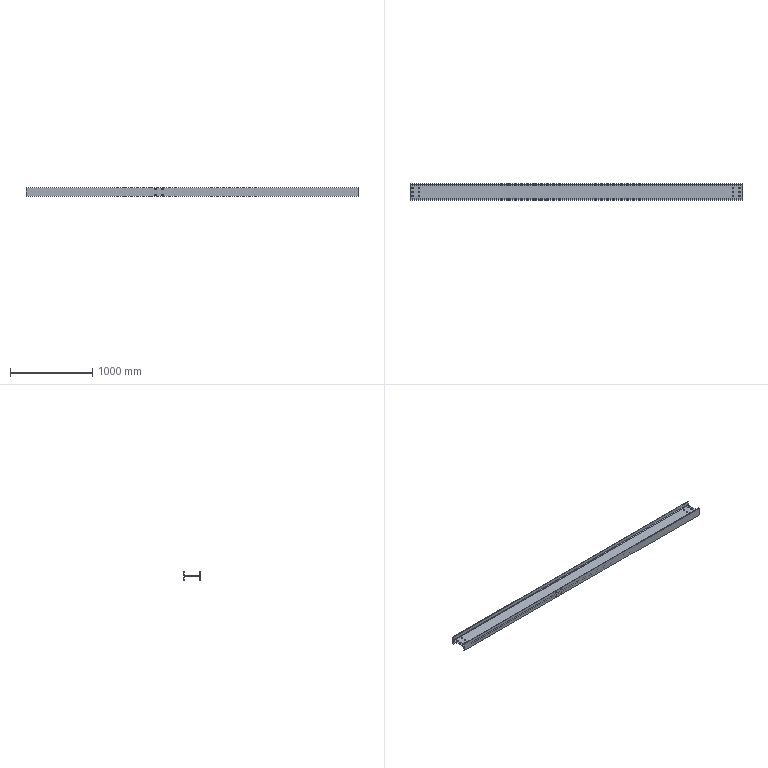Part | STEP file | 计量主梁3主体_Default<As Machined> | 1 solid | 58 faces | box 4030 x 200 x 100 mm | volume 10713895 mm3 | cylinder 36 | plane 22 | commonest cylinder face diameters 19 x32 16 x4